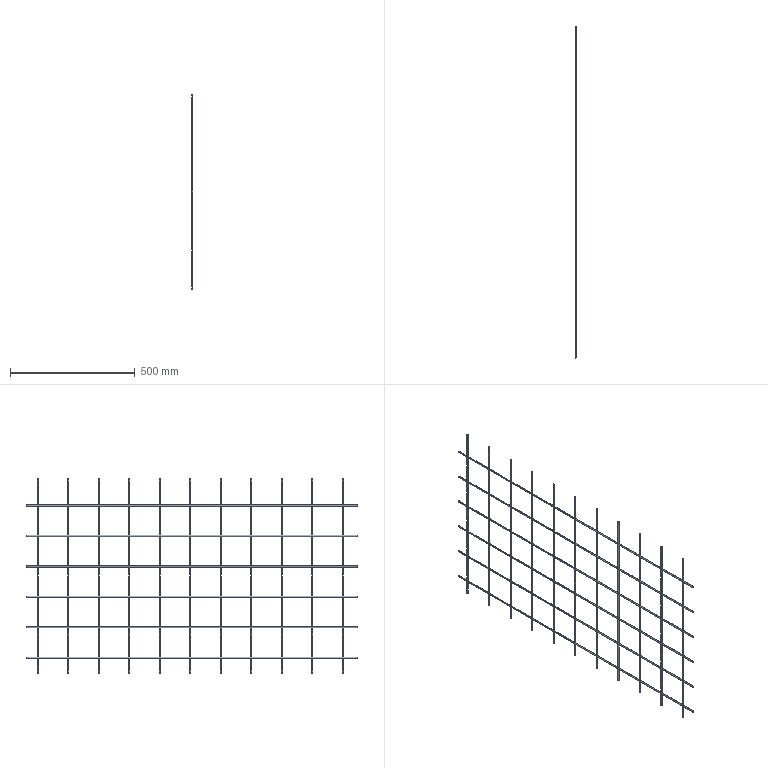Part | SolidWorks | features BaseBody 1, ICE 1, MirrorPattern 1 | 1 solid | 68 faces | box 8 x 1328 x 777 mm | volume 322628 mm3 | cylinder 34 | plane 34 | commonest cylinder face diameters 5 x34